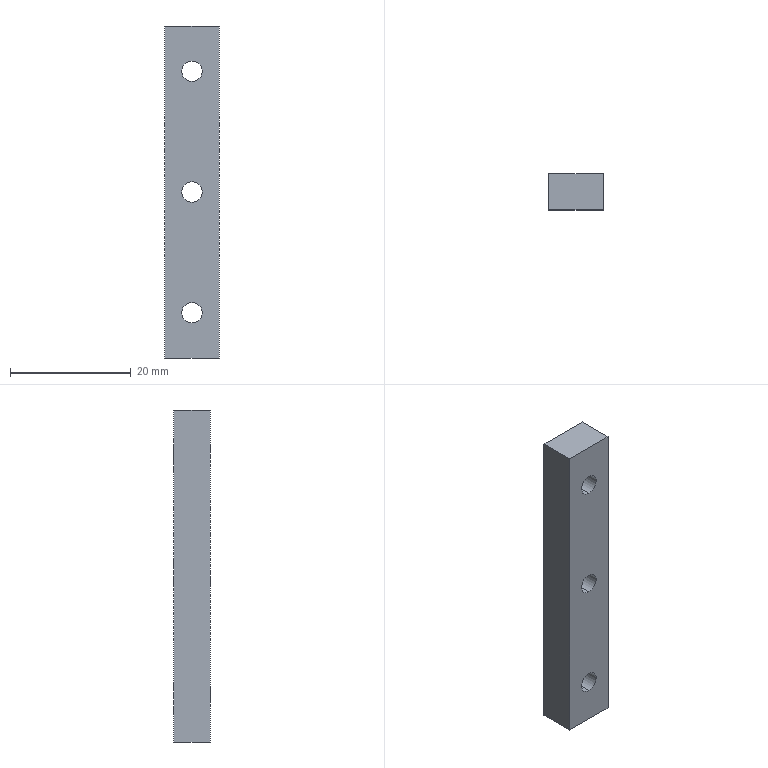Part | STEP file | 1 solid | 21 faces | box 9 x 6 x 55 mm | volume 2652 mm3 | cylinder 12 | plane 9 | commonest cylinder face diameters 3.4 x6 5.5 x6